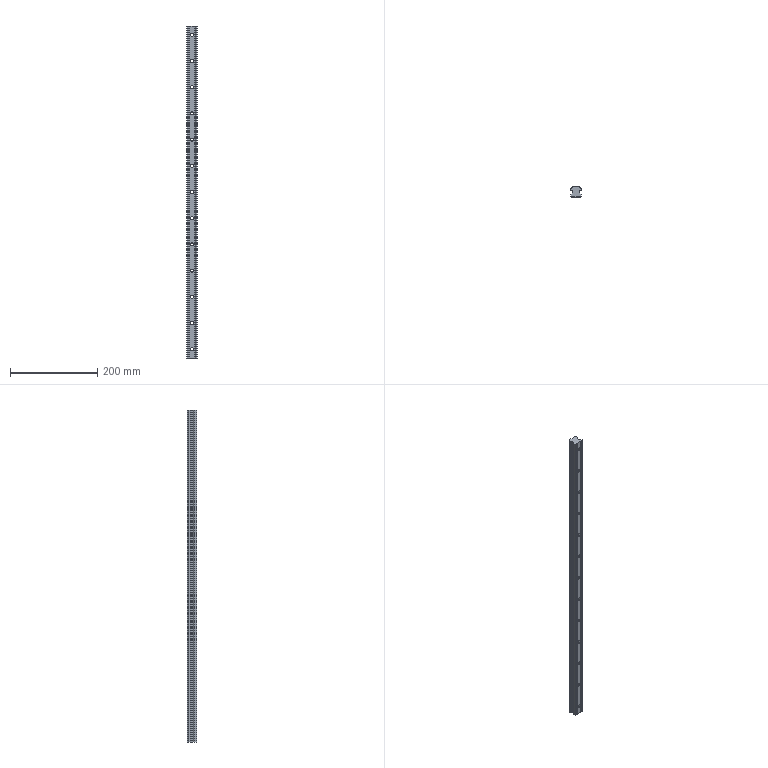Part | STEP file | HGR25R760C Guide Rail | 1 solid | 99 faces | box 23 x 22 x 760 mm | volume 316727 mm3 | cylinder 56 | plane 43 | commonest cylinder face diameters 7 x26 11 x26 4.6 x4